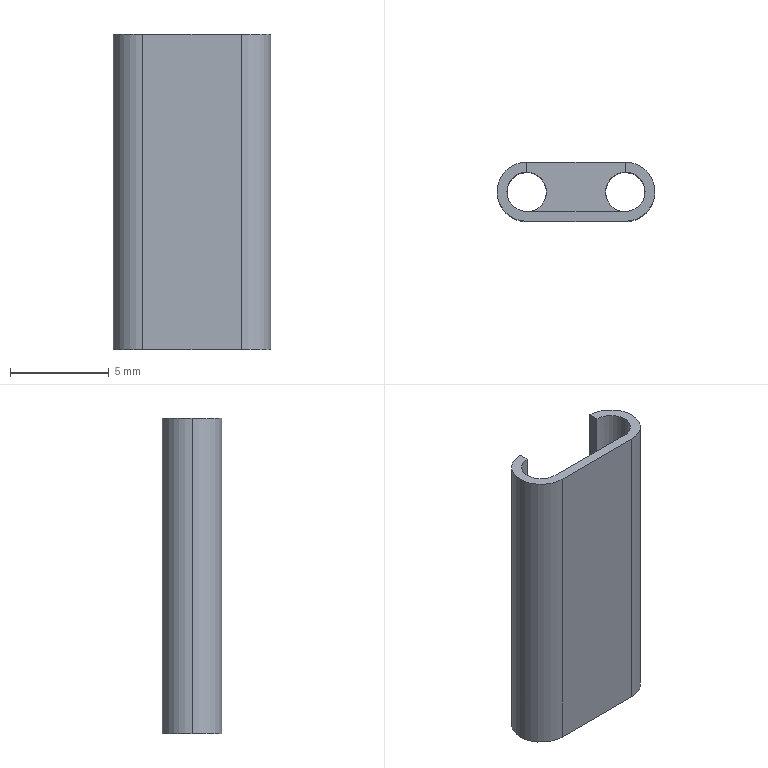Part | STEP file | 102000006971 | 1 solid | 16 faces | box 8 x 3 x 16 mm | volume 158.982 mm3 | cylinder 8 | plane 8 | commonest cylinder face diameters 2 x4 3 x4
STEP:
#1=CARTESIAN_POINT('',(-2.5,-1.,6.));
#2=VERTEX_POINT('',#1);
#3=CARTESIAN_POINT('',(-1.5,0.,6.));
#4=VERTEX_POINT('',#3);
#5=CARTESIAN_POINT('',(-2.5,0.,6.));
#6=DIRECTION('',(0.,0.,-1.));
#7=AXIS2_PLACEMENT_3D('',#5,#6,$);
#8=CIRCLE('',#7,1.);
#9=EDGE_CURVE('',#2,#4,#8,.F.);
#10=ORIENTED_EDGE('',*,*,#9,.T.);
#11=CARTESIAN_POINT('',(-1.5,0.,0.));
#12=VERTEX_POINT('',#11);
#13=CARTESIAN_POINT('',(-1.5,0.,16.));
#14=DIRECTION('',(0.,0.,-1.));
#15=VECTOR('',#14,1.);
#16=LINE('',#13,#15);
#17=EDGE_CURVE('',#4,#12,#16,.T.);
#18=ORIENTED_EDGE('',*,*,#17,.T.);
#19=CARTESIAN_POINT('',(-3.5,0.,0.));
#20=VERTEX_POINT('',#19);
#21=CARTESIAN_POINT('',(-2.5,0.,0.));
#22=DIRECTION('',(0.,0.,-1.));
#23=AXIS2_PLACEMENT_3D('',#21,#22,$);
#24=CIRCLE('',#23,1.);
#25=EDGE_CURVE('',#20,#12,#24,.F.);
#26=ORIENTED_EDGE('',*,*,#25,.F.);
#27=CARTESIAN_POINT('',(-3.5,0.,16.));
#28=VERTEX_POINT('',#27);
#29=CARTESIAN_POINT('',(-3.5,0.,16.));
#30=DIRECTION('',(0.,0.,-1.));
#31=VECTOR('',#30,1.);
#32=LINE('',#29,#31);
#33=EDGE_CURVE('',#28,#20,#32,.T.);
#34=ORIENTED_EDGE('',*,*,#33,.F.);
#35=CARTESIAN_POINT('',(-2.5,-1.,16.));
#36=VERTEX_POINT('',#35);
#37=CARTESIAN_POINT('',(-2.5,0.,16.));
#38=DIRECTION('',(0.,0.,-1.));
#39=AXIS2_PLACEMENT_3D('',#37,#38,$);
#40=CIRCLE('',#39,1.);
#41=EDGE_CURVE('',#28,#36,#40,.F.);
#42=ORIENTED_EDGE('',*,*,#41,.T.);
#43=CARTESIAN_POINT('',(-2.5,-1.,16.));
#44=DIRECTION('',(0.,0.,-1.));
#45=VECTOR('',#44,1.);
#46=LINE('',#43,#45);
#47=EDGE_CURVE('',#2,#36,#46,.F.);
#48=ORIENTED_EDGE('',*,*,#47,.F.);
#49=EDGE_LOOP('',(#10,#18,#26,#34,#42,#48));
#50=FACE_OUTER_BOUND('',#49,.T.);
#51=CARTESIAN_POINT('',(-2.5,0.,16.));
#52=DIRECTION('',(0.,0.,-1.));
#53=DIRECTION('',(1.,0.,0.));
#54=AXIS2_PLACEMENT_3D('',#51,#52,#53);
#55=CYLINDRICAL_SURFACE('',#54,1.);
#56=ADVANCED_FACE('',(#50),#55,.F.);
#57=CARTESIAN_POINT('',(2.5,1.,6.));
#58=VERTEX_POINT('',#57);
#59=CARTESIAN_POINT('',(2.5,1.5,6.));
#60=VERTEX_POINT('',#59);
#61=CARTESIAN_POINT('',(2.5,1.25,6.));
#62=DIRECTION('',(0.,1.,0.));
#63=VECTOR('',#62,1.);
#64=LINE('',#61,#63);
#65=EDGE_CURVE('',#58,#60,#64,.T.);
#66=ORIENTED_EDGE('',*,*,#65,.T.);
#67=CARTESIAN_POINT('',(-2.5,1.5,6.));
#68=VERTEX_POINT('',#67);
#69=CARTESIAN_POINT('',(0.,1.5,6.));
#70=DIRECTION('',(-1.,0.,0.));
#71=VECTOR('',#70,1.);
#72=LINE('',#69,#71);
#73=EDGE_CURVE('',#60,#68,#72,.T.);
#74=ORIENTED_EDGE('',*,*,#73,.T.);
#75=CARTESIAN_POINT('',(-2.5,1.,6.));
#76=VERTEX_POINT('',#75);
#77=CARTESIAN_POINT('',(-2.5,1.25,6.));
#78=DIRECTION('',(0.,-1.,0.));
#79=VECTOR('',#78,1.);
#80=LINE('',#77,#79);
#81=EDGE_CURVE('',#68,#76,#80,.T.);
#82=ORIENTED_EDGE('',*,*,#81,.T.);
#83=CARTESIAN_POINT('',(-2.5,-0.000000003,6.));
#84=DIRECTION('',(0.,0.,1.));
#85=AXIS2_PLACEMENT_3D('',#83,#84,$);
#86=CIRCLE('',#85,1.);
#87=EDGE_CURVE('',#4,#76,#86,.T.);
#88=ORIENTED_EDGE('',*,*,#87,.F.);
#89=ORIENTED_EDGE('',*,*,#9,.F.);
#90=CARTESIAN_POINT('',(2.5,-1.,6.));
#91=VERTEX_POINT('',#90);
#92=CARTESIAN_POINT('',(0.,-1.,6.));
#93=DIRECTION('',(1.,0.,0.));
#94=VECTOR('',#93,1.);
#95=LINE('',#92,#94);
#96=EDGE_CURVE('',#2,#91,#95,.T.);
#97=ORIENTED_EDGE('',*,*,#96,.T.);
#98=CARTESIAN_POINT('',(1.5,0.,6.));
#99=VERTEX_POINT('',#98);
#100=CARTESIAN_POINT('',(2.5,0.000000003,6.));
#101=DIRECTION('',(0.,0.,1.));
#102=AXIS2_PLACEMENT_3D('',#100,#101,$);
#103=CIRCLE('',#102,1.);
#104=EDGE_CURVE('',#99,#91,#103,.T.);
#105=ORIENTED_EDGE('',*,*,#104,.F.);
#106=CARTESIAN_POINT('',(2.5,-0.000000003,6.));
#107=DIRECTION('',(0.,0.,1.));
#108=AXIS2_PLACEMENT_3D('',#106,#107,$);
#109=CIRCLE('',#108,1.);
#110=EDGE_CURVE('',#58,#99,#109,.T.);
#111=ORIENTED_EDGE('',*,*,#110,.F.);
#112=EDGE_LOOP('',(#66,#74,#82,#88,#89,#97,#105,#111));
#113=FACE_OUTER_BOUND('',#112,.T.);
#114=CARTESIAN_POINT('',(0.,0.,6.));
#115=DIRECTION('',(0.,0.,1.));
#116=DIRECTION('',(1.,0.,0.));
#117=AXIS2_PLACEMENT_3D('',#114,#115,#116);
#118=PLANE('',#117);
#119=ADVANCED_FACE('',(#113),#118,.T.);
#120=ORIENTED_EDGE('',*,*,#17,.F.);
#121=ORIENTED_EDGE('',*,*,#87,.T.);
#122=CARTESIAN_POINT('',(-2.5,1.,16.));
#123=VERTEX_POINT('',#122);
#124=CARTESIAN_POINT('',(-2.5,1.,16.));
#125=DIRECTION('',(0.,0.,-1.));
#126=VECTOR('',#125,1.);
#127=LINE('',#124,#126);
#128=EDGE_CURVE('',#123,#76,#127,.T.);
#129=ORIENTED_EDGE('',*,*,#128,.F.);
#130=CARTESIAN_POINT('',(-2.5,0.,16.));
#131=DIRECTION('',(0.,0.,-1.));
#132=AXIS2_PLACEMENT_3D('',#130,#131,$);
#133=CIRCLE('',#132,1.);
#134=EDGE_CURVE('',#123,#28,#133,.F.);
#135=ORIENTED_EDGE('',*,*,#134,.T.);
#136=ORIENTED_EDGE('',*,*,#33,.T.);
#137=CARTESIAN_POINT('',(-2.5,0.,0.));
#138=DIRECTION('',(0.,0.,-1.));
#139=AXIS2_PLACEMENT_3D('',#137,#138,$);
#140=CIRCLE('',#139,1.);
#141=EDGE_CURVE('',#12,#20,#140,.F.);
#142=ORIENTED_EDGE('',*,*,#141,.F.);
#143=EDGE_LOOP('',(#120,#121,#129,#135,#136,#142));
#144=FACE_OUTER_BOUND('',#143,.T.);
#145=CARTESIAN_POINT('',(-2.5,0.,16.));
#146=DIRECTION('',(0.,0.,-1.));
#147=DIRECTION('',(-1.,0.,0.));
#148=AXIS2_PLACEMENT_3D('',#145,#146,#147);
#149=CYLINDRICAL_SURFACE('',#148,1.);
#150=ADVANCED_FACE('',(#144),#149,.F.);
#151=CARTESIAN_POINT('',(4.,0.,0.));
#152=VERTEX_POINT('',#151);
#153=CARTESIAN_POINT('',(2.5,1.5,0.));
#154=VERTEX_POINT('',#153);
#155=CARTESIAN_POINT('',(2.5,0.,0.));
#156=DIRECTION('',(0.,0.,1.));
#157=AXIS2_PLACEMENT_3D('',#155,#156,$);
#158=CIRCLE('',#157,1.5);
#159=EDGE_CURVE('',#152,#154,#158,.T.);
#160=ORIENTED_EDGE('',*,*,#159,.F.);
#161=CARTESIAN_POINT('',(2.5,-1.5,0.));
#162=VERTEX_POINT('',#161);
#163=CARTESIAN_POINT('',(2.5,0.,0.));
#164=DIRECTION('',(0.,0.,1.));
#165=AXIS2_PLACEMENT_3D('',#163,#164,$);
#166=CIRCLE('',#165,1.5);
#167=EDGE_CURVE('',#162,#152,#166,.T.);
#168=ORIENTED_EDGE('',*,*,#167,.F.);
#169=CARTESIAN_POINT('',(-2.5,-1.5,0.));
#170=VERTEX_POINT('',#169);
#171=CARTESIAN_POINT('',(0.,-1.5,0.));
#172=DIRECTION('',(1.,0.,0.));
#173=VECTOR('',#172,1.);
#174=LINE('',#171,#173);
#175=EDGE_CURVE('',#170,#162,#174,.T.);
#176=ORIENTED_EDGE('',*,*,#175,.F.);
#177=CARTESIAN_POINT('',(-4.,0.,0.));
#178=VERTEX_POINT('',#177);
#179=CARTESIAN_POINT('',(-2.5,-0.000000002,0.));
#180=DIRECTION('',(0.,0.,1.));
#181=AXIS2_PLACEMENT_3D('',#179,#180,$);
#182=CIRCLE('',#181,1.5);
#183=EDGE_CURVE('',#178,#170,#182,.T.);
#184=ORIENTED_EDGE('',*,*,#183,.F.);
#185=CARTESIAN_POINT('',(-2.5,1.5,0.));
#186=VERTEX_POINT('',#185);
#187=CARTESIAN_POINT('',(-2.5,0.000000002,0.));
#188=DIRECTION('',(0.,0.,1.));
#189=AXIS2_PLACEMENT_3D('',#187,#188,$);
#190=CIRCLE('',#189,1.5);
#191=EDGE_CURVE('',#186,#178,#190,.T.);
#192=ORIENTED_EDGE('',*,*,#191,.F.);
#193=CARTESIAN_POINT('',(0.,1.5,0.));
#194=DIRECTION('',(-1.,0.,0.));
#195=VECTOR('',#194,1.);
#196=LINE('',#193,#195);
#197=EDGE_CURVE('',#154,#186,#196,.T.);
#198=ORIENTED_EDGE('',*,*,#197,.F.);
#199=EDGE_LOOP('',(#160,#168,#176,#184,#192,#198));
#200=FACE_OUTER_BOUND('',#199,.T.);
#201=CARTESIAN_POINT('',(1.5,0.,0.));
#202=VERTEX_POINT('',#201);
#203=CARTESIAN_POINT('',(3.5,0.,0.));
#204=VERTEX_POINT('',#203);
#205=CARTESIAN_POINT('',(2.5,0.,0.));
#206=DIRECTION('',(0.,0.,1.));
#207=AXIS2_PLACEMENT_3D('',#205,#206,$);
#208=CIRCLE('',#207,1.);
#209=EDGE_CURVE('',#202,#204,#208,.T.);
#210=ORIENTED_EDGE('',*,*,#209,.T.);
#211=CARTESIAN_POINT('',(2.5,0.,0.));
#212=DIRECTION('',(0.,0.,1.));
#213=AXIS2_PLACEMENT_3D('',#211,#212,$);
#214=CIRCLE('',#213,1.);
#215=EDGE_CURVE('',#204,#202,#214,.T.);
#216=ORIENTED_EDGE('',*,*,#215,.T.);
#217=EDGE_LOOP('',(#210,#216));
#218=FACE_BOUND('',#217,.T.);
#219=ORIENTED_EDGE('',*,*,#25,.T.);
#220=ORIENTED_EDGE('',*,*,#141,.T.);
#221=EDGE_LOOP('',(#219,#220));
#222=FACE_BOUND('',#221,.T.);
#223=CARTESIAN_POINT('',(2.5,0.,0.));
#224=DIRECTION('',(0.,0.,1.));
#225=DIRECTION('',(1.,0.,0.));
#226=AXIS2_PLACEMENT_3D('',#223,#224,#225);
#227=PLANE('',#226);
#228=ADVANCED_FACE('',(#200,#218,#222),#227,.F.);
#229=CARTESIAN_POINT('',(2.5,1.,16.));
#230=VERTEX_POINT('',#229);
#231=CARTESIAN_POINT('',(2.5,1.5,16.));
#232=VERTEX_POINT('',#231);
#233=CARTESIAN_POINT('',(2.5,1.25,16.));
#234=DIRECTION('',(0.,1.,0.));
#235=VECTOR('',#234,1.);
#236=LINE('',#233,#235);
#237=EDGE_CURVE('',#230,#232,#236,.T.);
#238=ORIENTED_EDGE('',*,*,#237,.F.);
#239=CARTESIAN_POINT('',(3.5,0.,16.));
#240=VERTEX_POINT('',#239);
#241=CARTESIAN_POINT('',(2.5,-0.000000003,16.));
#242=DIRECTION('',(0.,0.,1.));
#243=AXIS2_PLACEMENT_3D('',#241,#242,$);
#244=CIRCLE('',#243,1.);
#245=EDGE_CURVE('',#240,#230,#244,.T.);
#246=ORIENTED_EDGE('',*,*,#245,.F.);
#247=CARTESIAN_POINT('',(2.5,-1.,16.));
#248=VERTEX_POINT('',#247);
#249=CARTESIAN_POINT('',(2.5,0.000000003,16.));
#250=DIRECTION('',(0.,0.,1.));
#251=AXIS2_PLACEMENT_3D('',#249,#250,$);
#252=CIRCLE('',#251,1.);
#253=EDGE_CURVE('',#248,#240,#252,.T.);
#254=ORIENTED_EDGE('',*,*,#253,.F.);
#255=CARTESIAN_POINT('',(0.,-1.,16.));
#256=DIRECTION('',(1.,0.,0.));
#257=VECTOR('',#256,1.);
#258=LINE('',#255,#257);
#259=EDGE_CURVE('',#36,#248,#258,.T.);
#260=ORIENTED_EDGE('',*,*,#259,.F.);
#261=ORIENTED_EDGE('',*,*,#41,.F.);
#262=ORIENTED_EDGE('',*,*,#134,.F.);
#263=CARTESIAN_POINT('',(-2.5,1.5,16.));
#264=VERTEX_POINT('',#263);
#265=CARTESIAN_POINT('',(-2.5,1.25,16.));
#266=DIRECTION('',(0.,-1.,0.));
#267=VECTOR('',#266,1.);
#268=LINE('',#265,#267);
#269=EDGE_CURVE('',#264,#123,#268,.T.);
#270=ORIENTED_EDGE('',*,*,#269,.F.);
#271=CARTESIAN_POINT('',(-4.,0.,16.));
#272=VERTEX_POINT('',#271);
#273=CARTESIAN_POINT('',(-2.5,0.000000002,16.));
#274=DIRECTION('',(0.,0.,1.));
#275=AXIS2_PLACEMENT_3D('',#273,#274,$);
#276=CIRCLE('',#275,1.5);
#277=EDGE_CURVE('',#264,#272,#276,.T.);
#278=ORIENTED_EDGE('',*,*,#277,.T.);
#279=CARTESIAN_POINT('',(-2.5,-1.5,16.));
#280=VERTEX_POINT('',#279);
#281=CARTESIAN_POINT('',(-2.5,-0.000000002,16.));
#282=DIRECTION('',(0.,0.,1.));
#283=AXIS2_PLACEMENT_3D('',#281,#282,$);
#284=CIRCLE('',#283,1.5);
#285=EDGE_CURVE('',#272,#280,#284,.T.);
#286=ORIENTED_EDGE('',*,*,#285,.T.);
#287=CARTESIAN_POINT('',(2.5,-1.5,16.));
#288=VERTEX_POINT('',#287);
#289=CARTESIAN_POINT('',(0.,-1.5,16.));
#290=DIRECTION('',(1.,0.,0.));
#291=VECTOR('',#290,1.);
#292=LINE('',#289,#291);
#293=EDGE_CURVE('',#280,#288,#292,.T.);
#294=ORIENTED_EDGE('',*,*,#293,.T.);
#295=CARTESIAN_POINT('',(4.,0.,16.));
#296=VERTEX_POINT('',#295);
#297=CARTESIAN_POINT('',(2.5,0.,16.));
#298=DIRECTION('',(0.,0.,1.));
#299=AXIS2_PLACEMENT_3D('',#297,#298,$);
#300=CIRCLE('',#299,1.5);
#301=EDGE_CURVE('',#288,#296,#300,.T.);
#302=ORIENTED_EDGE('',*,*,#301,.T.);
#303=CARTESIAN_POINT('',(2.5,0.,16.));
#304=DIRECTION('',(0.,0.,1.));
#305=AXIS2_PLACEMENT_3D('',#303,#304,$);
#306=CIRCLE('',#305,1.5);
#307=EDGE_CURVE('',#296,#232,#306,.T.);
#308=ORIENTED_EDGE('',*,*,#307,.T.);
#309=EDGE_LOOP('',(#238,#246,#254,#260,#261,#262,#270,#278,#286,#294,#302,#308));
#310=FACE_OUTER_BOUND('',#309,.T.);
#311=CARTESIAN_POINT('',(2.5,0.,16.));
#312=DIRECTION('',(0.,0.,1.));
#313=DIRECTION('',(1.,0.,0.));
#314=AXIS2_PLACEMENT_3D('',#311,#312,#313);
#315=PLANE('',#314);
#316=ADVANCED_FACE('',(#310),#315,.T.);
#317=ORIENTED_EDGE('',*,*,#259,.T.);
#318=CARTESIAN_POINT('',(2.5,-1.,11.));
#319=DIRECTION('',(0.,0.,1.));
#320=VECTOR('',#319,1.);
#321=LINE('',#318,#320);
#322=EDGE_CURVE('',#91,#248,#321,.T.);
#323=ORIENTED_EDGE('',*,*,#322,.F.);
#324=ORIENTED_EDGE('',*,*,#96,.F.);
#325=ORIENTED_EDGE('',*,*,#47,.T.);
#326=EDGE_LOOP('',(#317,#323,#324,#325));
#327=FACE_OUTER_BOUND('',#326,.T.);
#328=CARTESIAN_POINT('',(-2.5,-1.,6.));
#329=DIRECTION('',(0.,-1.,0.));
#330=DIRECTION('',(0.,0.,-1.));
#331=AXIS2_PLACEMENT_3D('',#328,#329,#330);
#332=PLANE('',#331);
#333=ADVANCED_FACE('',(#327),#332,.F.);
#334=CARTESIAN_POINT('',(2.5,1.,11.));
#335=DIRECTION('',(0.,0.,1.));
#336=VECTOR('',#335,1.);
#337=LINE('',#334,#336);
#338=EDGE_CURVE('',#58,#230,#337,.T.);
#339=ORIENTED_EDGE('',*,*,#338,.T.);
#340=ORIENTED_EDGE('',*,*,#237,.T.);
#341=CARTESIAN_POINT('',(2.5,1.5,11.));
#342=DIRECTION('',(0.,0.,-1.));
#343=VECTOR('',#342,1.);
#344=LINE('',#341,#343);
#345=EDGE_CURVE('',#232,#60,#344,.T.);
#346=ORIENTED_EDGE('',*,*,#345,.T.);
#347=ORIENTED_EDGE('',*,*,#65,.F.);
#348=EDGE_LOOP('',(#339,#340,#346,#347));
#349=FACE_OUTER_BOUND('',#348,.T.);
#350=CARTESIAN_POINT('',(2.5,-1.,6.));
#351=DIRECTION('',(1.,0.,0.));
#352=DIRECTION('',(0.,0.,-1.));
#353=AXIS2_PLACEMENT_3D('',#350,#351,#352);
#354=PLANE('',#353);
#355=ADVANCED_FACE('',(#349),#354,.F.);
#356=ORIENTED_EDGE('',*,*,#73,.F.);
#357=CARTESIAN_POINT('',(2.5,1.5,3.));
#358=DIRECTION('',(0.,0.,-1.));
#359=VECTOR('',#358,1.);
#360=LINE('',#357,#359);
#361=EDGE_CURVE('',#60,#154,#360,.T.);
#362=ORIENTED_EDGE('',*,*,#361,.T.);
#363=ORIENTED_EDGE('',*,*,#197,.T.);
#364=CARTESIAN_POINT('',(-2.5,1.5,3.));
#365=DIRECTION('',(0.,0.,-1.));
#366=VECTOR('',#365,1.);
#367=LINE('',#364,#366);
#368=EDGE_CURVE('',#68,#186,#367,.T.);
#369=ORIENTED_EDGE('',*,*,#368,.F.);
#370=EDGE_LOOP('',(#356,#362,#363,#369));
#371=FACE_OUTER_BOUND('',#370,.T.);
#372=CARTESIAN_POINT('',(-2.5,1.5,16.));
#373=DIRECTION('',(0.,-1.,0.));
#374=DIRECTION('',(0.,0.,-1.));
#375=AXIS2_PLACEMENT_3D('',#372,#373,#374);
#376=PLANE('',#375);
#377=ADVANCED_FACE('',(#371),#376,.F.);
#378=ORIENTED_EDGE('',*,*,#128,.T.);
#379=ORIENTED_EDGE('',*,*,#81,.F.);
#380=CARTESIAN_POINT('',(-2.5,1.5,11.));
#381=DIRECTION('',(0.,0.,-1.));
#382=VECTOR('',#381,1.);
#383=LINE('',#380,#382);
#384=EDGE_CURVE('',#264,#68,#383,.T.);
#385=ORIENTED_EDGE('',*,*,#384,.F.);
#386=ORIENTED_EDGE('',*,*,#269,.T.);
#387=EDGE_LOOP('',(#378,#379,#385,#386));
#388=FACE_OUTER_BOUND('',#387,.T.);
#389=CARTESIAN_POINT('',(-2.5,1.5,6.));
#390=DIRECTION('',(-1.,0.,0.));
#391=DIRECTION('',(0.,0.,1.));
#392=AXIS2_PLACEMENT_3D('',#389,#390,#391);
#393=PLANE('',#392);
#394=ADVANCED_FACE('',(#388),#393,.F.);
#395=ORIENTED_EDGE('',*,*,#253,.T.);
#396=CARTESIAN_POINT('',(3.5,0.,16.));
#397=DIRECTION('',(0.,0.,-1.));
#398=VECTOR('',#397,1.);
#399=LINE('',#396,#398);
#400=EDGE_CURVE('',#240,#204,#399,.T.);
#401=ORIENTED_EDGE('',*,*,#400,.T.);
#402=ORIENTED_EDGE('',*,*,#209,.F.);
#403=CARTESIAN_POINT('',(1.5,0.,16.));
#404=DIRECTION('',(0.,0.,-1.));
#405=VECTOR('',#404,1.);
#406=LINE('',#403,#405);
#407=EDGE_CURVE('',#99,#202,#406,.T.);
#408=ORIENTED_EDGE('',*,*,#407,.F.);
#409=ORIENTED_EDGE('',*,*,#104,.T.);
#410=ORIENTED_EDGE('',*,*,#322,.T.);
#411=EDGE_LOOP('',(#395,#401,#402,#408,#409,#410));
#412=FACE_OUTER_BOUND('',#411,.T.);
#413=CARTESIAN_POINT('',(2.5,0.,16.));
#414=DIRECTION('',(0.,0.,-1.));
#415=DIRECTION('',(1.,0.,0.));
#416=AXIS2_PLACEMENT_3D('',#413,#414,#415);
#417=CYLINDRICAL_SURFACE('',#416,1.);
#418=ADVANCED_FACE('',(#412),#417,.F.);
#419=ORIENTED_EDGE('',*,*,#400,.F.);
#420=ORIENTED_EDGE('',*,*,#245,.T.);
#421=ORIENTED_EDGE('',*,*,#338,.F.);
#422=ORIENTED_EDGE('',*,*,#110,.T.);
#423=ORIENTED_EDGE('',*,*,#407,.T.);
#424=ORIENTED_EDGE('',*,*,#215,.F.);
#425=EDGE_LOOP('',(#419,#420,#421,#422,#423,#424));
#426=FACE_OUTER_BOUND('',#425,.T.);
#427=CARTESIAN_POINT('',(2.5,0.,16.));
#428=DIRECTION('',(0.,0.,-1.));
#429=DIRECTION('',(-1.,0.,0.));
#430=AXIS2_PLACEMENT_3D('',#427,#428,#429);
#431=CYLINDRICAL_SURFACE('',#430,1.);
#432=ADVANCED_FACE('',(#426),#431,.F.);
#433=CARTESIAN_POINT('',(4.,0.,16.));
#434=DIRECTION('',(0.,0.,-1.));
#435=VECTOR('',#434,1.);
#436=LINE('',#433,#435);
#437=EDGE_CURVE('',#296,#152,#436,.T.);
#438=ORIENTED_EDGE('',*,*,#437,.T.);
#439=ORIENTED_EDGE('',*,*,#159,.T.);
#440=ORIENTED_EDGE('',*,*,#361,.F.);
#441=ORIENTED_EDGE('',*,*,#345,.F.);
#442=ORIENTED_EDGE('',*,*,#307,.F.);
#443=EDGE_LOOP('',(#438,#439,#440,#441,#442));
#444=FACE_OUTER_BOUND('',#443,.T.);
#445=CARTESIAN_POINT('',(2.5,0.,16.));
#446=DIRECTION('',(0.,0.,-1.));
#447=DIRECTION('',(-1.,0.,0.));
#448=AXIS2_PLACEMENT_3D('',#445,#446,#447);
#449=CYLINDRICAL_SURFACE('',#448,1.5);
#450=ADVANCED_FACE('',(#444),#449,.T.);
#451=ORIENTED_EDGE('',*,*,#437,.F.);
#452=ORIENTED_EDGE('',*,*,#301,.F.);
#453=CARTESIAN_POINT('',(2.5,-1.5,16.));
#454=DIRECTION('',(0.,0.,-1.));
#455=VECTOR('',#454,1.);
#456=LINE('',#453,#455);
#457=EDGE_CURVE('',#288,#162,#456,.T.);
#458=ORIENTED_EDGE('',*,*,#457,.T.);
#459=ORIENTED_EDGE('',*,*,#167,.T.);
#460=EDGE_LOOP('',(#451,#452,#458,#459));
#461=FACE_OUTER_BOUND('',#460,.T.);
#462=CARTESIAN_POINT('',(2.5,0.,16.));
#463=DIRECTION('',(0.,0.,-1.));
#464=DIRECTION('',(1.,0.,0.));
#465=AXIS2_PLACEMENT_3D('',#462,#463,#464);
#466=CYLINDRICAL_SURFACE('',#465,1.5);
#467=ADVANCED_FACE('',(#461),#466,.T.);
#468=ORIENTED_EDGE('',*,*,#175,.T.);
#469=ORIENTED_EDGE('',*,*,#457,.F.);
#470=ORIENTED_EDGE('',*,*,#293,.F.);
#471=CARTESIAN_POINT('',(-2.5,-1.5,8.));
#472=DIRECTION('',(0.,0.,-1.));
#473=VECTOR('',#472,1.);
#474=LINE('',#471,#473);
#475=EDGE_CURVE('',#280,#170,#474,.T.);
#476=ORIENTED_EDGE('',*,*,#475,.T.);
#477=EDGE_LOOP('',(#468,#469,#470,#476));
#478=FACE_OUTER_BOUND('',#477,.T.);
#479=CARTESIAN_POINT('',(-2.5,-1.5,16.));
#480=DIRECTION('',(0.,1.,0.));
#481=DIRECTION('',(0.,0.,1.));
#482=AXIS2_PLACEMENT_3D('',#479,#480,#481);
#483=PLANE('',#482);
#484=ADVANCED_FACE('',(#478),#483,.F.);
#485=ORIENTED_EDGE('',*,*,#285,.F.);
#486=CARTESIAN_POINT('',(-4.,0.,16.));
#487=DIRECTION('',(0.,0.,-1.));
#488=VECTOR('',#487,1.);
#489=LINE('',#486,#488);
#490=EDGE_CURVE('',#272,#178,#489,.T.);
#491=ORIENTED_EDGE('',*,*,#490,.T.);
#492=ORIENTED_EDGE('',*,*,#183,.T.);
#493=ORIENTED_EDGE('',*,*,#475,.F.);
#494=EDGE_LOOP('',(#485,#491,#492,#493));
#495=FACE_OUTER_BOUND('',#494,.T.);
#496=CARTESIAN_POINT('',(-2.5,0.,16.));
#497=DIRECTION('',(0.,0.,-1.));
#498=DIRECTION('',(1.,0.,0.));
#499=AXIS2_PLACEMENT_3D('',#496,#497,#498);
#500=CYLINDRICAL_SURFACE('',#499,1.5);
#501=ADVANCED_FACE('',(#495),#500,.T.);
#502=ORIENTED_EDGE('',*,*,#490,.F.);
#503=ORIENTED_EDGE('',*,*,#277,.F.);
#504=ORIENTED_EDGE('',*,*,#384,.T.);
#505=ORIENTED_EDGE('',*,*,#368,.T.);
#506=ORIENTED_EDGE('',*,*,#191,.T.);
#507=EDGE_LOOP('',(#502,#503,#504,#505,#506));
#508=FACE_OUTER_BOUND('',#507,.T.);
#509=CARTESIAN_POINT('',(-2.5,0.,16.));
#510=DIRECTION('',(0.,0.,-1.));
#511=DIRECTION('',(-1.,0.,0.));
#512=AXIS2_PLACEMENT_3D('',#509,#510,#511);
#513=CYLINDRICAL_SURFACE('',#512,1.5);
#514=ADVANCED_FACE('',(#508),#513,.T.);
#515=CLOSED_SHELL('',(#56,#119,#150,#228,#316,#333,#355,#377,#394,#418,#432,#450,#467,#484,#501,#514));
#516=MANIFOLD_SOLID_BREP('',#515);
#517=(LENGTH_UNIT()NAMED_UNIT(*)SI_UNIT(.MILLI.,.METRE.));
#518=UNCERTAINTY_MEASURE_WITH_UNIT(LENGTH_MEASURE(0.005),#517,'','');
#519=(NAMED_UNIT(*)PLANE_ANGLE_UNIT()SI_UNIT($,.RADIAN.));
#520=(NAMED_UNIT(*)SI_UNIT($,.STERADIAN.)SOLID_ANGLE_UNIT());
#521=(GEOMETRIC_REPRESENTATION_CONTEXT(3)GLOBAL_UNCERTAINTY_ASSIGNED_CONTEXT((#518))GLOBAL_UNIT_ASSIGNED_CONTEXT((#517,#519,#520))REPRESENTATION_CONTEXT('',''));
#522=ADVANCED_BREP_SHAPE_REPRESENTATION('',(#516),#521);